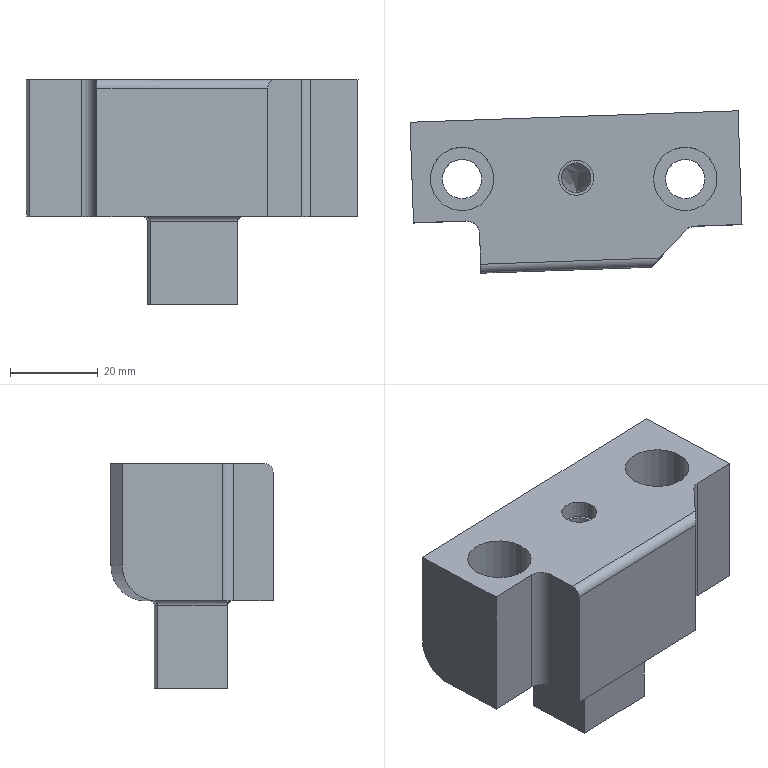Part | NX | features DIE-78 2 | 1 solid | 33 faces | box 75.862 x 37.072 x 51.4 mm | volume 69934 mm3 | plane 18 | cylinder 14 | cone 1 | commonest cylinder face diameters 2 x4 6 x2 9 x2 14.5 x2 4 x1 6.806 x1
STEP:
#1=CARTESIAN_POINT('',(3783.039,-805.598,860.616));
#2=VERTEX_POINT('',#1);
#3=CARTESIAN_POINT('',(3783.284,-812.594,860.616));
#4=VERTEX_POINT('',#3);
#5=CARTESIAN_POINT('',(3784.202,-838.885,860.616));
#6=DIRECTION('',(-0.0349,0.9994,0.));
#7=VECTOR('',#6,1000.);
#8=LINE('',#5,#7);
#9=EDGE_CURVE('',#2,#4,#8,.F.);
#10=ORIENTED_EDGE('',*,*,#9,.T.);
#11=CARTESIAN_POINT('',(3824.259,-811.163,860.616));
#12=VERTEX_POINT('',#11);
#13=CARTESIAN_POINT('',(3833.719,-810.833,860.616));
#14=DIRECTION('',(-0.9994,-0.0349,0.));
#15=VECTOR('',#14,1000.);
#16=LINE('',#13,#15);
#17=EDGE_CURVE('',#4,#12,#16,.F.);
#18=ORIENTED_EDGE('',*,*,#17,.T.);
#19=CARTESIAN_POINT('',(3830.163,-804.832,860.616));
#20=VERTEX_POINT('',#19);
#21=CARTESIAN_POINT('',(3816.137,-819.872,860.616));
#22=DIRECTION('',(0.682,0.7314,0.));
#23=VECTOR('',#22,1000.);
#24=LINE('',#21,#23);
#25=EDGE_CURVE('',#12,#20,#24,.T.);
#26=ORIENTED_EDGE('',*,*,#25,.T.);
#27=CARTESIAN_POINT('',(3832.252,-803.88,860.616));
#28=VERTEX_POINT('',#27);
#29=CARTESIAN_POINT('',(3832.357,-806.878,860.616));
#30=DIRECTION('',(0.,0.,-1.));
#31=DIRECTION('',(-1.,0.,0.));
#32=AXIS2_PLACEMENT_3D('',#29,#30,#31);
#33=CIRCLE('',#32,3.);
#34=EDGE_CURVE('',#20,#28,#33,.T.);
#35=ORIENTED_EDGE('',*,*,#34,.T.);
#36=CARTESIAN_POINT('',(3843.003,-803.505,860.616));
#37=VERTEX_POINT('',#36);
#38=CARTESIAN_POINT('',(3833.475,-803.837,860.616));
#39=DIRECTION('',(-0.9994,-0.0349,0.));
#40=VECTOR('',#39,1000.);
#41=LINE('',#38,#40);
#42=EDGE_CURVE('',#28,#37,#41,.F.);
#43=ORIENTED_EDGE('',*,*,#42,.T.);
#44=CARTESIAN_POINT('',(3842.096,-777.521,860.616));
#45=VERTEX_POINT('',#44);
#46=CARTESIAN_POINT('',(3842.011,-775.091,860.616));
#47=DIRECTION('',(0.0349,-0.9994,0.));
#48=VECTOR('',#47,1000.);
#49=LINE('',#46,#48);
#50=EDGE_CURVE('',#37,#45,#49,.F.);
#51=ORIENTED_EDGE('',*,*,#50,.T.);
#52=CARTESIAN_POINT('',(3767.141,-780.138,860.616));
#53=VERTEX_POINT('',#52);
#54=CARTESIAN_POINT('',(3832.568,-777.853,860.616));
#55=DIRECTION('',(-0.9994,-0.0349,0.));
#56=VECTOR('',#55,1000.);
#57=LINE('',#54,#56);
#58=EDGE_CURVE('',#53,#45,#57,.F.);
#59=ORIENTED_EDGE('',*,*,#58,.F.);
#60=CARTESIAN_POINT('',(3767.944,-803.124,860.616));
#61=VERTEX_POINT('',#60);
#62=CARTESIAN_POINT('',(3767.056,-777.709,860.616));
#63=DIRECTION('',(-0.0349,0.9994,0.));
#64=VECTOR('',#63,1000.);
#65=LINE('',#62,#64);
#66=EDGE_CURVE('',#53,#61,#65,.F.);
#67=ORIENTED_EDGE('',*,*,#66,.T.);
#68=CARTESIAN_POINT('',(3779.937,-802.705,860.616));
#69=VERTEX_POINT('',#68);
#70=CARTESIAN_POINT('',(3833.37,-800.839,860.616));
#71=DIRECTION('',(-0.9994,-0.0349,0.));
#72=VECTOR('',#71,1000.);
#73=LINE('',#70,#72);
#74=EDGE_CURVE('',#61,#69,#73,.F.);
#75=ORIENTED_EDGE('',*,*,#74,.T.);
#76=CARTESIAN_POINT('',(3780.041,-805.703,860.616));
#77=DIRECTION('',(0.,0.,-1.));
#78=DIRECTION('',(-1.,0.,0.));
#79=AXIS2_PLACEMENT_3D('',#76,#77,#78);
#80=CIRCLE('',#79,3.);
#81=EDGE_CURVE('',#69,#2,#80,.T.);
#82=ORIENTED_EDGE('',*,*,#81,.T.);
#83=EDGE_LOOP('',(#10,#18,#26,#35,#43,#51,#59,#67,#75,#82));
#84=FACE_BOUND('',#83,.T.);
#85=CARTESIAN_POINT('',(3771.787,-793.095,860.616));
#86=VERTEX_POINT('',#85);
#87=CARTESIAN_POINT('',(3779.037,-793.095,860.616));
#88=DIRECTION('',(0.,0.,-1.));
#89=DIRECTION('',(-1.,0.,0.));
#90=AXIS2_PLACEMENT_3D('',#87,#88,#89);
#91=CIRCLE('',#90,7.25);
#92=EDGE_CURVE('',#86,#86,#91,.F.);
#93=ORIENTED_EDGE('',*,*,#92,.F.);
#94=EDGE_LOOP('',(#93));
#95=FACE_BOUND('',#94,.T.);
#96=CARTESIAN_POINT('',(3822.787,-793.095,860.616));
#97=VERTEX_POINT('',#96);
#98=CARTESIAN_POINT('',(3830.037,-793.095,860.616));
#99=DIRECTION('',(0.,0.,-1.));
#100=DIRECTION('',(-1.,0.,0.));
#101=AXIS2_PLACEMENT_3D('',#98,#99,#100);
#102=CIRCLE('',#101,7.25);
#103=EDGE_CURVE('',#97,#97,#102,.F.);
#104=ORIENTED_EDGE('',*,*,#103,.F.);
#105=EDGE_LOOP('',(#104));
#106=FACE_BOUND('',#105,.T.);
#107=CARTESIAN_POINT('',(3809.107,-792.821,860.616));
#108=VERTEX_POINT('',#107);
#109=CARTESIAN_POINT('',(3805.107,-792.821,860.616));
#110=DIRECTION('',(0.,0.,-1.));
#111=DIRECTION('',(1.,0.,0.));
#112=AXIS2_PLACEMENT_3D('',#109,#110,#111);
#113=CIRCLE('',#112,4.);
#114=EDGE_CURVE('',#108,#108,#113,.T.);
#115=ORIENTED_EDGE('',*,*,#114,.T.);
#116=EDGE_LOOP('',(#115));
#117=FACE_BOUND('',#116,.T.);
#118=CARTESIAN_POINT('',(3834.637,-837.124,860.616));
#119=DIRECTION('',(0.,0.,-1.));
#120=DIRECTION('',(0.,-1.,0.));
#121=AXIS2_PLACEMENT_3D('',#118,#119,#120);
#122=PLANE('',#121);
#123=ADVANCED_FACE('',(#84,#95,#106,#117),#122,.F.);
#124=CARTESIAN_POINT('',(3767.42,-788.133,829.216));
#125=VERTEX_POINT('',#124);
#126=CARTESIAN_POINT('',(3767.141,-780.138,837.216));
#127=VERTEX_POINT('',#126);
#128=CARTESIAN_POINT('',(3767.42,-788.133,837.216));
#129=DIRECTION('',(0.9994,0.0349,0.000000002));
#130=DIRECTION('',(-0.0349,0.9994,0.));
#131=AXIS2_PLACEMENT_3D('',#128,#129,#130);
#132=CIRCLE('',#131,8.);
#133=EDGE_CURVE('',#125,#127,#132,.T.);
#134=ORIENTED_EDGE('',*,*,#133,.T.);
#135=CARTESIAN_POINT('',(3842.096,-777.521,837.216));
#136=VERTEX_POINT('',#135);
#137=CARTESIAN_POINT('',(3827.105,-778.044,837.216));
#138=DIRECTION('',(0.9994,0.0349,0.));
#139=VECTOR('',#138,1000.);
#140=LINE('',#137,#139);
#141=EDGE_CURVE('',#127,#136,#140,.T.);
#142=ORIENTED_EDGE('',*,*,#141,.T.);
#143=CARTESIAN_POINT('',(3842.375,-785.516,829.216));
#144=VERTEX_POINT('',#143);
#145=CARTESIAN_POINT('',(3842.375,-785.516,837.216));
#146=DIRECTION('',(-0.9994,-0.0349,-0.000000002));
#147=DIRECTION('',(0.0349,-0.9994,0.));
#148=AXIS2_PLACEMENT_3D('',#145,#146,#147);
#149=CIRCLE('',#148,8.);
#150=EDGE_CURVE('',#136,#144,#149,.T.);
#151=ORIENTED_EDGE('',*,*,#150,.T.);
#152=CARTESIAN_POINT('',(3815.891,-786.44,829.216));
#153=VERTEX_POINT('',#152);
#154=CARTESIAN_POINT('',(3782.411,-787.609,829.216));
#155=DIRECTION('',(0.9994,0.0349,0.));
#156=VECTOR('',#155,1000.);
#157=LINE('',#154,#156);
#158=EDGE_CURVE('',#153,#144,#157,.T.);
#159=ORIENTED_EDGE('',*,*,#158,.F.);
#160=CARTESIAN_POINT('',(3793.904,-787.208,829.216));
#161=VERTEX_POINT('',#160);
#162=CARTESIAN_POINT('',(3782.411,-787.609,829.216));
#163=DIRECTION('',(0.9994,0.0349,0.));
#164=VECTOR('',#163,1000.);
#165=LINE('',#162,#164);
#166=EDGE_CURVE('',#161,#153,#165,.T.);
#167=ORIENTED_EDGE('',*,*,#166,.F.);
#168=CARTESIAN_POINT('',(3782.411,-787.609,829.216));
#169=DIRECTION('',(0.9994,0.0349,0.));
#170=VECTOR('',#169,1000.);
#171=LINE('',#168,#170);
#172=EDGE_CURVE('',#125,#161,#171,.T.);
#173=ORIENTED_EDGE('',*,*,#172,.F.);
#174=EDGE_LOOP('',(#134,#142,#151,#159,#167,#173));
#175=FACE_BOUND('',#174,.T.);
#176=CARTESIAN_POINT('',(3782.411,-787.609,837.216));
#177=DIRECTION('',(0.9994,0.0349,0.000000002));
#178=DIRECTION('',(-0.0349,0.9994,0.));
#179=AXIS2_PLACEMENT_3D('',#176,#177,#178);
#180=CYLINDRICAL_SURFACE('',#179,8.);
#181=ADVANCED_FACE('',(#175),#180,.T.);
#182=ORIENTED_EDGE('',*,*,#81,.F.);
#183=CARTESIAN_POINT('',(3779.937,-802.705,829.216));
#184=VERTEX_POINT('',#183);
#185=CARTESIAN_POINT('',(3779.937,-802.705,860.616));
#186=DIRECTION('',(0.,0.000000057,-1.));
#187=VECTOR('',#186,1000.);
#188=LINE('',#185,#187);
#189=EDGE_CURVE('',#184,#69,#188,.F.);
#190=ORIENTED_EDGE('',*,*,#189,.F.);
#191=CARTESIAN_POINT('',(3783.039,-805.598,829.216));
#192=VERTEX_POINT('',#191);
#193=CARTESIAN_POINT('',(3780.041,-805.703,829.216));
#194=DIRECTION('',(0.,0.,-1.));
#195=DIRECTION('',(-1.,0.,0.));
#196=AXIS2_PLACEMENT_3D('',#193,#194,#195);
#197=CIRCLE('',#196,3.);
#198=EDGE_CURVE('',#192,#184,#197,.F.);
#199=ORIENTED_EDGE('',*,*,#198,.F.);
#200=CARTESIAN_POINT('',(3783.039,-805.598,829.216));
#201=DIRECTION('',(0.,0.000000057,-1.));
#202=VECTOR('',#201,1000.);
#203=LINE('',#200,#202);
#204=EDGE_CURVE('',#2,#192,#203,.T.);
#205=ORIENTED_EDGE('',*,*,#204,.F.);
#206=EDGE_LOOP('',(#182,#190,#199,#205));
#207=FACE_BOUND('',#206,.T.);
#208=CARTESIAN_POINT('',(3780.041,-805.703,842.216));
#209=DIRECTION('',(0.,-0.000000057,1.));
#210=DIRECTION('',(0.,-1.,-0.000000057));
#211=AXIS2_PLACEMENT_3D('',#208,#209,#210);
#212=CYLINDRICAL_SURFACE('',#211,3.);
#213=ADVANCED_FACE('',(#207),#212,.F.);
#214=CARTESIAN_POINT('',(3767.944,-803.124,829.216));
#215=VERTEX_POINT('',#214);
#216=CARTESIAN_POINT('',(3040.928,-828.509,829.216));
#217=DIRECTION('',(-0.9994,-0.0349,0.));
#218=VECTOR('',#217,1000.);
#219=LINE('',#216,#218);
#220=EDGE_CURVE('',#184,#215,#219,.T.);
#221=ORIENTED_EDGE('',*,*,#220,.F.);
#222=ORIENTED_EDGE('',*,*,#189,.T.);
#223=ORIENTED_EDGE('',*,*,#74,.F.);
#224=CARTESIAN_POINT('',(3767.944,-803.124,842.216));
#225=DIRECTION('',(0.,-0.000000057,1.));
#226=VECTOR('',#225,1000.);
#227=LINE('',#224,#226);
#228=EDGE_CURVE('',#215,#61,#227,.T.);
#229=ORIENTED_EDGE('',*,*,#228,.F.);
#230=EDGE_LOOP('',(#221,#222,#223,#229));
#231=FACE_BOUND('',#230,.T.);
#232=CARTESIAN_POINT('',(3835.403,-800.768,844.916));
#233=DIRECTION('',(0.0349,-0.9994,-0.000000057));
#234=DIRECTION('',(0.9994,0.0349,0.));
#235=AXIS2_PLACEMENT_3D('',#232,#233,#234);
#236=PLANE('',#235);
#237=ADVANCED_FACE('',(#231),#236,.T.);
#238=CARTESIAN_POINT('',(3767.056,-777.709,829.216));
#239=DIRECTION('',(-0.0349,0.9994,0.));
#240=VECTOR('',#239,1000.);
#241=LINE('',#238,#240);
#242=EDGE_CURVE('',#125,#215,#241,.F.);
#243=ORIENTED_EDGE('',*,*,#242,.T.);
#244=ORIENTED_EDGE('',*,*,#228,.T.);
#245=ORIENTED_EDGE('',*,*,#66,.F.);
#246=CARTESIAN_POINT('',(3767.141,-780.138,823.716));
#247=DIRECTION('',(0.,-0.000000057,1.));
#248=VECTOR('',#247,1000.);
#249=LINE('',#246,#248);
#250=EDGE_CURVE('',#127,#53,#249,.T.);
#251=ORIENTED_EDGE('',*,*,#250,.F.);
#252=ORIENTED_EDGE('',*,*,#133,.F.);
#253=EDGE_LOOP('',(#243,#244,#245,#251,#252));
#254=FACE_BOUND('',#253,.T.);
#255=CARTESIAN_POINT('',(3767.056,-777.709,842.216));
#256=DIRECTION('',(-0.9994,-0.0349,-0.000000002));
#257=DIRECTION('',(-0.0349,0.9994,0.));
#258=AXIS2_PLACEMENT_3D('',#255,#256,#257);
#259=PLANE('',#258);
#260=ADVANCED_FACE('',(#254),#259,.T.);
#261=ORIENTED_EDGE('',*,*,#141,.F.);
#262=ORIENTED_EDGE('',*,*,#250,.T.);
#263=ORIENTED_EDGE('',*,*,#58,.T.);
#264=CARTESIAN_POINT('',(3842.096,-777.521,823.716));
#265=DIRECTION('',(0.,0.000000057,-1.));
#266=VECTOR('',#265,1000.);
#267=LINE('',#264,#266);
#268=EDGE_CURVE('',#45,#136,#267,.T.);
#269=ORIENTED_EDGE('',*,*,#268,.T.);
#270=EDGE_LOOP('',(#261,#262,#263,#269));
#271=FACE_BOUND('',#270,.T.);
#272=CARTESIAN_POINT('',(3789.628,-779.353,823.716));
#273=DIRECTION('',(0.0349,-0.9994,-0.000000057));
#274=DIRECTION('',(-0.9994,-0.0349,0.));
#275=AXIS2_PLACEMENT_3D('',#272,#273,#274);
#276=PLANE('',#275);
#277=ADVANCED_FACE('',(#271),#276,.F.);
#278=ORIENTED_EDGE('',*,*,#50,.F.);
#279=CARTESIAN_POINT('',(3843.003,-803.505,829.216));
#280=VERTEX_POINT('',#279);
#281=CARTESIAN_POINT('',(3843.003,-803.505,842.216));
#282=DIRECTION('',(0.,0.000000057,-1.));
#283=VECTOR('',#282,1000.);
#284=LINE('',#281,#283);
#285=EDGE_CURVE('',#37,#280,#284,.T.);
#286=ORIENTED_EDGE('',*,*,#285,.T.);
#287=CARTESIAN_POINT('',(3842.011,-775.091,829.216));
#288=DIRECTION('',(0.0349,-0.9994,0.));
#289=VECTOR('',#288,1000.);
#290=LINE('',#287,#289);
#291=EDGE_CURVE('',#280,#144,#290,.F.);
#292=ORIENTED_EDGE('',*,*,#291,.T.);
#293=ORIENTED_EDGE('',*,*,#150,.F.);
#294=ORIENTED_EDGE('',*,*,#268,.F.);
#295=EDGE_LOOP('',(#278,#286,#292,#293,#294));
#296=FACE_BOUND('',#295,.T.);
#297=CARTESIAN_POINT('',(3842.011,-775.091,842.216));
#298=DIRECTION('',(0.9994,0.0349,0.000000002));
#299=DIRECTION('',(0.0349,-0.9994,0.));
#300=AXIS2_PLACEMENT_3D('',#297,#298,#299);
#301=PLANE('',#300);
#302=ADVANCED_FACE('',(#296),#301,.T.);
#303=ORIENTED_EDGE('',*,*,#42,.F.);
#304=CARTESIAN_POINT('',(3832.252,-803.88,829.216));
#305=VERTEX_POINT('',#304);
#306=CARTESIAN_POINT('',(3832.252,-803.88,829.216));
#307=DIRECTION('',(0.,-0.000000057,1.));
#308=VECTOR('',#307,1000.);
#309=LINE('',#306,#308);
#310=EDGE_CURVE('',#28,#305,#309,.F.);
#311=ORIENTED_EDGE('',*,*,#310,.T.);
#312=CARTESIAN_POINT('',(3828.012,-804.028,829.216));
#313=DIRECTION('',(0.9994,0.0349,0.));
#314=VECTOR('',#313,1000.);
#315=LINE('',#312,#314);
#316=EDGE_CURVE('',#305,#280,#315,.T.);
#317=ORIENTED_EDGE('',*,*,#316,.T.);
#318=ORIENTED_EDGE('',*,*,#285,.F.);
#319=EDGE_LOOP('',(#303,#311,#317,#318));
#320=FACE_BOUND('',#319,.T.);
#321=CARTESIAN_POINT('',(3828.012,-804.028,842.216));
#322=DIRECTION('',(0.0349,-0.9994,-0.000000057));
#323=DIRECTION('',(0.,0.000000057,-1.));
#324=AXIS2_PLACEMENT_3D('',#321,#322,#323);
#325=PLANE('',#324);
#326=ADVANCED_FACE('',(#320),#325,.T.);
#327=ORIENTED_EDGE('',*,*,#34,.F.);
#328=CARTESIAN_POINT('',(3830.163,-804.832,829.216));
#329=VERTEX_POINT('',#328);
#330=CARTESIAN_POINT('',(3830.163,-804.832,860.616));
#331=DIRECTION('',(0.,0.000000057,-1.));
#332=VECTOR('',#331,1000.);
#333=LINE('',#330,#332);
#334=EDGE_CURVE('',#329,#20,#333,.F.);
#335=ORIENTED_EDGE('',*,*,#334,.F.);
#336=CARTESIAN_POINT('',(3832.357,-806.878,829.216));
#337=DIRECTION('',(0.,0.,-1.));
#338=DIRECTION('',(-1.,0.,0.));
#339=AXIS2_PLACEMENT_3D('',#336,#337,#338);
#340=CIRCLE('',#339,3.);
#341=EDGE_CURVE('',#305,#329,#340,.F.);
#342=ORIENTED_EDGE('',*,*,#341,.F.);
#343=ORIENTED_EDGE('',*,*,#310,.F.);
#344=EDGE_LOOP('',(#327,#335,#342,#343));
#345=FACE_BOUND('',#344,.T.);
#346=CARTESIAN_POINT('',(3832.357,-806.878,842.216));
#347=DIRECTION('',(0.,0.000000057,-1.));
#348=DIRECTION('',(0.,1.,0.000000057));
#349=AXIS2_PLACEMENT_3D('',#346,#347,#348);
#350=CYLINDRICAL_SURFACE('',#349,3.);
#351=ADVANCED_FACE('',(#345),#350,.F.);
#352=CARTESIAN_POINT('',(3825.537,-793.095,829.216));
#353=VERTEX_POINT('',#352);
#354=CARTESIAN_POINT('',(3830.037,-793.095,829.216));
#355=DIRECTION('',(0.,0.,-1.));
#356=DIRECTION('',(-1.,0.,0.));
#357=AXIS2_PLACEMENT_3D('',#354,#355,#356);
#358=CIRCLE('',#357,4.5);
#359=EDGE_CURVE('',#353,#353,#358,.T.);
#360=ORIENTED_EDGE('',*,*,#359,.F.);
#361=EDGE_LOOP('',(#360));
#362=FACE_BOUND('',#361,.T.);
#363=CARTESIAN_POINT('',(3774.537,-793.095,829.216));
#364=VERTEX_POINT('',#363);
#365=CARTESIAN_POINT('',(3779.037,-793.095,829.216));
#366=DIRECTION('',(0.,0.,-1.));
#367=DIRECTION('',(-1.,0.,0.));
#368=AXIS2_PLACEMENT_3D('',#365,#366,#367);
#369=CIRCLE('',#368,4.5);
#370=EDGE_CURVE('',#364,#364,#369,.T.);
#371=ORIENTED_EDGE('',*,*,#370,.F.);
#372=EDGE_LOOP('',(#371));
#373=FACE_BOUND('',#372,.T.);
#374=CARTESIAN_POINT('',(3794.532,-805.197,829.216));
#375=VERTEX_POINT('',#374);
#376=CARTESIAN_POINT('',(3816.519,-804.429,829.216));
#377=VERTEX_POINT('',#376);
#378=CARTESIAN_POINT('',(3815.52,-804.464,829.216));
#379=DIRECTION('',(-0.9994,-0.0349,0.));
#380=VECTOR('',#379,1000.);
#381=LINE('',#378,#380);
#382=EDGE_CURVE('',#375,#377,#381,.F.);
#383=ORIENTED_EDGE('',*,*,#382,.T.);
#384=CARTESIAN_POINT('',(3815.682,-780.462,829.216));
#385=DIRECTION('',(-0.0349,0.9994,0.));
#386=VECTOR('',#385,1000.);
#387=LINE('',#384,#386);
#388=EDGE_CURVE('',#377,#153,#387,.T.);
#389=ORIENTED_EDGE('',*,*,#388,.T.);
#390=ORIENTED_EDGE('',*,*,#158,.T.);
#391=ORIENTED_EDGE('',*,*,#291,.F.);
#392=ORIENTED_EDGE('',*,*,#316,.F.);
#393=ORIENTED_EDGE('',*,*,#341,.T.);
#394=CARTESIAN_POINT('',(3822.33,-813.232,829.216));
#395=VERTEX_POINT('',#394);
#396=CARTESIAN_POINT('',(3461.379,-1200.302,829.216));
#397=DIRECTION('',(0.682,0.7314,0.));
#398=VECTOR('',#397,1000.);
#399=LINE('',#396,#398);
#400=EDGE_CURVE('',#329,#395,#399,.F.);
#401=ORIENTED_EDGE('',*,*,#400,.T.);
#402=CARTESIAN_POINT('',(3783.353,-814.593,829.216));
#403=VERTEX_POINT('',#402);
#404=CARTESIAN_POINT('',(3843.369,-812.497,829.216));
#405=DIRECTION('',(-0.9994,-0.0349,0.));
#406=VECTOR('',#405,1000.);
#407=LINE('',#404,#406);
#408=EDGE_CURVE('',#395,#403,#407,.T.);
#409=ORIENTED_EDGE('',*,*,#408,.T.);
#410=CARTESIAN_POINT('',(3782.203,-781.631,829.216));
#411=DIRECTION('',(0.0349,-0.9994,0.));
#412=VECTOR('',#411,1000.);
#413=LINE('',#410,#412);
#414=EDGE_CURVE('',#192,#403,#413,.T.);
#415=ORIENTED_EDGE('',*,*,#414,.F.);
#416=ORIENTED_EDGE('',*,*,#198,.T.);
#417=ORIENTED_EDGE('',*,*,#220,.T.);
#418=ORIENTED_EDGE('',*,*,#242,.F.);
#419=ORIENTED_EDGE('',*,*,#172,.T.);
#420=CARTESIAN_POINT('',(3794.498,-804.198,829.216));
#421=DIRECTION('',(-0.0349,0.9994,0.));
#422=VECTOR('',#421,1000.);
#423=LINE('',#420,#422);
#424=EDGE_CURVE('',#161,#375,#423,.F.);
#425=ORIENTED_EDGE('',*,*,#424,.T.);
#426=EDGE_LOOP('',(#383,#389,#390,#391,#392,#393,#401,#409,#415,#416,#417,#418,#419,#425));
#427=FACE_BOUND('',#426,.T.);
#428=CARTESIAN_POINT('',(3040.196,-807.539,829.216));
#429=DIRECTION('',(0.,0.,-1.));
#430=DIRECTION('',(0.0349,-0.9994,0.));
#431=AXIS2_PLACEMENT_3D('',#428,#429,#430);
#432=PLANE('',#431);
#433=ADVANCED_FACE('',(#362,#373,#427),#432,.T.);
#434=ORIENTED_EDGE('',*,*,#25,.F.);
#435=CARTESIAN_POINT('',(3822.33,-813.232,858.616));
#436=VERTEX_POINT('',#435);
#437=CARTESIAN_POINT('',(3824.259,-811.163,858.616));
#438=DIRECTION('',(-0.7314,0.682,0.000000039));
#439=DIRECTION('',(0.682,0.7314,0.000000039));
#440=AXIS2_PLACEMENT_3D('',#437,#438,#439);
#441=ELLIPSE('',#440,2.828,2.);
#442=EDGE_CURVE('',#12,#436,#441,.F.);
#443=ORIENTED_EDGE('',*,*,#442,.T.);
#444=CARTESIAN_POINT('',(3822.33,-813.232,854.74));
#445=DIRECTION('',(0.,-0.000000057,1.));
#446=VECTOR('',#445,1000.);
#447=LINE('',#444,#446);
#448=EDGE_CURVE('',#395,#436,#447,.T.);
#449=ORIENTED_EDGE('',*,*,#448,.F.);
#450=ORIENTED_EDGE('',*,*,#400,.F.);
#451=ORIENTED_EDGE('',*,*,#334,.T.);
#452=EDGE_LOOP('',(#434,#443,#449,#450,#451));
#453=FACE_BOUND('',#452,.T.);
#454=CARTESIAN_POINT('',(3822.33,-813.232,854.74));
#455=DIRECTION('',(-0.7314,0.682,0.000000039));
#456=DIRECTION('',(0.,-0.000000057,1.));
#457=AXIS2_PLACEMENT_3D('',#454,#455,#456);
#458=PLANE('',#457);
#459=ADVANCED_FACE('',(#453),#458,.F.);
#460=CARTESIAN_POINT('',(3783.353,-814.593,858.616));
#461=VERTEX_POINT('',#460);
#462=CARTESIAN_POINT('',(3783.353,-814.593,842.216));
#463=DIRECTION('',(0.,0.000000057,-1.));
#464=VECTOR('',#463,1000.);
#465=LINE('',#462,#464);
#466=EDGE_CURVE('',#461,#403,#465,.T.);
#467=ORIENTED_EDGE('',*,*,#466,.F.);
#468=CARTESIAN_POINT('',(3783.284,-812.594,858.616));
#469=DIRECTION('',(-0.9994,-0.0349,-0.000000002));
#470=DIRECTION('',(0.0349,-0.9994,0.));
#471=AXIS2_PLACEMENT_3D('',#468,#469,#470);
#472=CIRCLE('',#471,2.);
#473=EDGE_CURVE('',#461,#4,#472,.T.);
#474=ORIENTED_EDGE('',*,*,#473,.T.);
#475=ORIENTED_EDGE('',*,*,#9,.F.);
#476=ORIENTED_EDGE('',*,*,#204,.T.);
#477=ORIENTED_EDGE('',*,*,#414,.T.);
#478=EDGE_LOOP('',(#467,#474,#475,#476,#477));
#479=FACE_BOUND('',#478,.T.);
#480=CARTESIAN_POINT('',(3782.047,-777.185,842.216));
#481=DIRECTION('',(-0.9994,-0.0349,-0.000000002));
#482=DIRECTION('',(-0.0349,0.9994,0.));
#483=AXIS2_PLACEMENT_3D('',#480,#481,#482);
#484=PLANE('',#483);
#485=ADVANCED_FACE('',(#479),#484,.T.);
#486=ORIENTED_EDGE('',*,*,#448,.T.);
#487=CARTESIAN_POINT('',(3843.369,-812.497,858.616));
#488=DIRECTION('',(0.9994,0.0349,0.));
#489=VECTOR('',#488,1000.);
#490=LINE('',#487,#489);
#491=EDGE_CURVE('',#436,#461,#490,.F.);
#492=ORIENTED_EDGE('',*,*,#491,.T.);
#493=ORIENTED_EDGE('',*,*,#466,.T.);
#494=ORIENTED_EDGE('',*,*,#408,.F.);
#495=EDGE_LOOP('',(#486,#492,#493,#494));
#496=FACE_BOUND('',#495,.T.);
#497=CARTESIAN_POINT('',(3843.369,-812.497,854.74));
#498=DIRECTION('',(0.0349,-0.9994,-0.000000057));
#499=DIRECTION('',(0.,-0.000000057,1.));
#500=AXIS2_PLACEMENT_3D('',#497,#498,#499);
#501=PLANE('',#500);
#502=ADVANCED_FACE('',(#496),#501,.T.);
#503=ORIENTED_EDGE('',*,*,#442,.F.);
#504=ORIENTED_EDGE('',*,*,#17,.F.);
#505=ORIENTED_EDGE('',*,*,#473,.F.);
#506=ORIENTED_EDGE('',*,*,#491,.F.);
#507=EDGE_LOOP('',(#503,#504,#505,#506));
#508=FACE_BOUND('',#507,.T.);
#509=CARTESIAN_POINT('',(3843.299,-810.499,858.616));
#510=DIRECTION('',(0.9994,0.0349,0.));
#511=DIRECTION('',(-0.0349,0.9994,0.));
#512=AXIS2_PLACEMENT_3D('',#509,#510,#511);
#513=CYLINDRICAL_SURFACE('',#512,2.);
#514=ADVANCED_FACE('',(#508),#513,.T.);
#515=CARTESIAN_POINT('',(3814.926,-787.475,809.216));
#516=VERTEX_POINT('',#515);
#517=CARTESIAN_POINT('',(3794.939,-788.173,809.216));
#518=VERTEX_POINT('',#517);
#519=CARTESIAN_POINT('',(3804.932,-787.824,809.216));
#520=DIRECTION('',(0.9994,0.0349,0.));
#521=VECTOR('',#520,1000.);
#522=LINE('',#519,#521);
#523=EDGE_CURVE('',#516,#518,#522,.F.);
#524=ORIENTED_EDGE('',*,*,#523,.F.);
#525=CARTESIAN_POINT('',(3815.485,-803.465,809.216));
#526=VERTEX_POINT('',#525);
#527=CARTESIAN_POINT('',(3815.485,-803.465,809.216));
#528=DIRECTION('',(-0.0349,0.9994,0.));
#529=VECTOR('',#528,1000.);
#530=LINE('',#527,#529);
#531=EDGE_CURVE('',#516,#526,#530,.F.);
#532=ORIENTED_EDGE('',*,*,#531,.T.);
#533=CARTESIAN_POINT('',(3795.497,-804.163,809.216));
#534=VERTEX_POINT('',#533);
#535=CARTESIAN_POINT('',(3805.491,-803.814,809.216));
#536=DIRECTION('',(0.9994,0.0349,0.));
#537=VECTOR('',#536,1000.);
#538=LINE('',#535,#537);
#539=EDGE_CURVE('',#526,#534,#538,.F.);
#540=ORIENTED_EDGE('',*,*,#539,.T.);
#541=CARTESIAN_POINT('',(3795.497,-804.163,809.216));
#542=DIRECTION('',(-0.0349,0.9994,0.));
#543=VECTOR('',#542,1000.);
#544=LINE('',#541,#543);
#545=EDGE_CURVE('',#518,#534,#544,.F.);
#546=ORIENTED_EDGE('',*,*,#545,.F.);
#547=EDGE_LOOP('',(#524,#532,#540,#546));
#548=FACE_BOUND('',#547,.T.);
#549=CARTESIAN_POINT('',(3804.689,-780.846,809.216));
#550=DIRECTION('',(0.,0.,1.));
#551=DIRECTION('',(-0.0349,0.9994,0.));
#552=AXIS2_PLACEMENT_3D('',#549,#550,#551);
#553=PLANE('',#552);
#554=ADVANCED_FACE('',(#548),#553,.F.);
#555=CARTESIAN_POINT('',(3815.485,-803.465,828.216));
#556=VERTEX_POINT('',#555);
#557=CARTESIAN_POINT('',(3815.485,-803.465,821.716));
#558=DIRECTION('',(0.,0.,-1.));
#559=VECTOR('',#558,1000.);
#560=LINE('',#557,#559);
#561=EDGE_CURVE('',#556,#526,#560,.T.);
#562=ORIENTED_EDGE('',*,*,#561,.F.);
#563=CARTESIAN_POINT('',(3795.497,-804.163,828.216));
#564=VERTEX_POINT('',#563);
#565=CARTESIAN_POINT('',(3795.497,-804.163,828.216));
#566=DIRECTION('',(-0.9994,-0.0349,0.));
#567=VECTOR('',#566,1000.);
#568=LINE('',#565,#567);
#569=EDGE_CURVE('',#556,#564,#568,.T.);
#570=ORIENTED_EDGE('',*,*,#569,.T.);
#571=CARTESIAN_POINT('',(3795.497,-804.163,814.216));
#572=DIRECTION('',(0.,0.,1.));
#573=VECTOR('',#572,1000.);
#574=LINE('',#571,#573);
#575=EDGE_CURVE('',#564,#534,#574,.F.);
#576=ORIENTED_EDGE('',*,*,#575,.T.);
#577=ORIENTED_EDGE('',*,*,#539,.F.);
#578=EDGE_LOOP('',(#562,#570,#576,#577));
#579=FACE_BOUND('',#578,.T.);
#580=CARTESIAN_POINT('',(3805.491,-803.814,821.716));
#581=DIRECTION('',(0.0349,-0.9994,0.));
#582=DIRECTION('',(0.,0.,1.));
#583=AXIS2_PLACEMENT_3D('',#580,#581,#582);
#584=PLANE('',#583);
#585=ADVANCED_FACE('',(#579),#584,.T.);
#586=CARTESIAN_POINT('',(3794.939,-788.173,828.216));
#587=VERTEX_POINT('',#586);
#588=CARTESIAN_POINT('',(3794.939,-788.173,814.216));
#589=DIRECTION('',(0.,0.,1.));
#590=VECTOR('',#589,1000.);
#591=LINE('',#588,#590);
#592=EDGE_CURVE('',#518,#587,#591,.T.);
#593=ORIENTED_EDGE('',*,*,#592,.T.);
#594=CARTESIAN_POINT('',(3814.926,-787.475,828.216));
#595=VERTEX_POINT('',#594);
#596=CARTESIAN_POINT('',(3814.926,-787.475,828.216));
#597=DIRECTION('',(-0.9994,-0.0349,0.));
#598=VECTOR('',#597,1000.);
#599=LINE('',#596,#598);
#600=EDGE_CURVE('',#587,#595,#599,.F.);
#601=ORIENTED_EDGE('',*,*,#600,.T.);
#602=CARTESIAN_POINT('',(3814.926,-787.475,814.216));
#603=DIRECTION('',(0.,0.,1.));
#604=VECTOR('',#603,1000.);
#605=LINE('',#602,#604);
#606=EDGE_CURVE('',#516,#595,#605,.T.);
#607=ORIENTED_EDGE('',*,*,#606,.F.);
#608=ORIENTED_EDGE('',*,*,#523,.T.);
#609=EDGE_LOOP('',(#593,#601,#607,#608));
#610=FACE_BOUND('',#609,.T.);
#611=CARTESIAN_POINT('',(3804.932,-787.824,814.216));
#612=DIRECTION('',(-0.0349,0.9994,0.));
#613=DIRECTION('',(0.,0.,-1.));
#614=AXIS2_PLACEMENT_3D('',#611,#612,#613);
#615=PLANE('',#614);
#616=ADVANCED_FACE('',(#610),#615,.T.);
#617=ORIENTED_EDGE('',*,*,#575,.F.);
#618=CARTESIAN_POINT('',(3794.904,-787.173,828.216));
#619=DIRECTION('',(-0.0349,0.9994,0.));
#620=VECTOR('',#619,1000.);
#621=LINE('',#618,#620);
#622=EDGE_CURVE('',#564,#587,#621,.T.);
#623=ORIENTED_EDGE('',*,*,#622,.T.);
#624=ORIENTED_EDGE('',*,*,#592,.F.);
#625=ORIENTED_EDGE('',*,*,#545,.T.);
#626=EDGE_LOOP('',(#617,#623,#624,#625));
#627=FACE_BOUND('',#626,.T.);
#628=CARTESIAN_POINT('',(3795.497,-804.163,814.216));
#629=DIRECTION('',(-0.9994,-0.0349,0.));
#630=DIRECTION('',(0.0349,-0.9994,0.));
#631=AXIS2_PLACEMENT_3D('',#628,#629,#630);
#632=PLANE('',#631);
#633=ADVANCED_FACE('',(#627),#632,.T.);
#634=ORIENTED_EDGE('',*,*,#606,.T.);
#635=CARTESIAN_POINT('',(3815.485,-803.465,828.216));
#636=DIRECTION('',(-0.0349,0.9994,0.));
#637=VECTOR('',#636,1000.);
#638=LINE('',#635,#637);
#639=EDGE_CURVE('',#595,#556,#638,.F.);
#640=ORIENTED_EDGE('',*,*,#639,.T.);
#641=ORIENTED_EDGE('',*,*,#561,.T.);
#642=ORIENTED_EDGE('',*,*,#531,.F.);
#643=EDGE_LOOP('',(#634,#640,#641,#642));
#644=FACE_BOUND('',#643,.T.);
#645=CARTESIAN_POINT('',(3815.485,-803.465,814.216));
#646=DIRECTION('',(-0.9994,-0.0349,0.));
#647=DIRECTION('',(0.0349,-0.9994,0.));
#648=AXIS2_PLACEMENT_3D('',#645,#646,#647);
#649=PLANE('',#648);
#650=ADVANCED_FACE('',(#644),#649,.F.);
#651=ORIENTED_EDGE('',*,*,#166,.T.);
#652=CARTESIAN_POINT('',(3815.891,-786.44,828.216));
#653=DIRECTION('',(0.7314,-0.682,0.));
#654=DIRECTION('',(0.682,0.7314,0.));
#655=AXIS2_PLACEMENT_3D('',#652,#653,#654);
#656=ELLIPSE('',#655,1.414,1.);
#657=EDGE_CURVE('',#153,#595,#656,.T.);
#658=ORIENTED_EDGE('',*,*,#657,.T.);
#659=ORIENTED_EDGE('',*,*,#600,.F.);
#660=CARTESIAN_POINT('',(3793.904,-787.208,828.216));
#661=DIRECTION('',(0.682,0.7314,0.));
#662=DIRECTION('',(0.7314,-0.682,0.));
#663=AXIS2_PLACEMENT_3D('',#660,#661,#662);
#664=ELLIPSE('',#663,1.414,1.);
#665=EDGE_CURVE('',#587,#161,#664,.F.);
#666=ORIENTED_EDGE('',*,*,#665,.T.);
#667=EDGE_LOOP('',(#651,#658,#659,#666));
#668=FACE_BOUND('',#667,.T.);
#669=CARTESIAN_POINT('',(3040.405,-813.518,828.216));
#670=DIRECTION('',(0.9994,0.0349,0.));
#671=DIRECTION('',(-0.0349,0.9994,0.));
#672=AXIS2_PLACEMENT_3D('',#669,#670,#671);
#673=CYLINDRICAL_SURFACE('',#672,1.);
#674=ADVANCED_FACE('',(#668),#673,.F.);
#675=ORIENTED_EDGE('',*,*,#665,.F.);
#676=ORIENTED_EDGE('',*,*,#622,.F.);
#677=CARTESIAN_POINT('',(3794.532,-805.197,828.216));
#678=DIRECTION('',(0.7314,-0.682,0.));
#679=DIRECTION('',(-0.682,-0.7314,0.));
#680=AXIS2_PLACEMENT_3D('',#677,#678,#679);
#681=ELLIPSE('',#680,1.414,1.);
#682=EDGE_CURVE('',#375,#564,#681,.F.);
#683=ORIENTED_EDGE('',*,*,#682,.F.);
#684=ORIENTED_EDGE('',*,*,#424,.F.);
#685=EDGE_LOOP('',(#675,#676,#683,#684));
#686=FACE_BOUND('',#685,.T.);
#687=CARTESIAN_POINT('',(3794.498,-804.198,828.216));
#688=DIRECTION('',(0.0349,-0.9994,0.));
#689=DIRECTION('',(0.9994,0.0349,0.));
#690=AXIS2_PLACEMENT_3D('',#687,#688,#689);
#691=CYLINDRICAL_SURFACE('',#690,1.);
#692=ADVANCED_FACE('',(#686),#691,.F.);
#693=ORIENTED_EDGE('',*,*,#682,.T.);
#694=ORIENTED_EDGE('',*,*,#569,.F.);
#695=CARTESIAN_POINT('',(3816.519,-804.429,828.216));
#696=DIRECTION('',(0.682,0.7314,0.));
#697=DIRECTION('',(0.7314,-0.682,0.));
#698=AXIS2_PLACEMENT_3D('',#695,#696,#697);
#699=ELLIPSE('',#698,1.414,1.);
#700=EDGE_CURVE('',#377,#556,#699,.F.);
#701=ORIENTED_EDGE('',*,*,#700,.F.);
#702=ORIENTED_EDGE('',*,*,#382,.F.);
#703=EDGE_LOOP('',(#693,#694,#701,#702));
#704=FACE_BOUND('',#703,.T.);
#705=CARTESIAN_POINT('',(3805.526,-804.813,828.216));
#706=DIRECTION('',(0.9994,0.0349,0.));
#707=DIRECTION('',(-0.0349,0.9994,0.));
#708=AXIS2_PLACEMENT_3D('',#705,#706,#707);
#709=CYLINDRICAL_SURFACE('',#708,1.);
#710=ADVANCED_FACE('',(#704),#709,.F.);
#711=ORIENTED_EDGE('',*,*,#700,.T.);
#712=ORIENTED_EDGE('',*,*,#639,.F.);
#713=ORIENTED_EDGE('',*,*,#657,.F.);
#714=ORIENTED_EDGE('',*,*,#388,.F.);
#715=EDGE_LOOP('',(#711,#712,#713,#714));
#716=FACE_BOUND('',#715,.T.);
#717=CARTESIAN_POINT('',(3815.682,-780.462,828.216));
#718=DIRECTION('',(-0.0349,0.9994,0.));
#719=DIRECTION('',(-0.9994,-0.0349,0.));
#720=AXIS2_PLACEMENT_3D('',#717,#718,#719);
#721=CYLINDRICAL_SURFACE('',#720,1.);
#722=ADVANCED_FACE('',(#716),#721,.F.);
#723=ORIENTED_EDGE('',*,*,#370,.T.);
#724=EDGE_LOOP('',(#723));
#725=FACE_BOUND('',#724,.T.);
#726=CARTESIAN_POINT('',(3783.537,-793.095,847.616));
#727=VERTEX_POINT('',#726);
#728=CARTESIAN_POINT('',(3779.037,-793.095,847.616));
#729=DIRECTION('',(0.,0.,1.));
#730=DIRECTION('',(1.,0.,0.));
#731=AXIS2_PLACEMENT_3D('',#728,#729,#730);
#732=CIRCLE('',#731,4.5);
#733=EDGE_CURVE('',#727,#727,#732,.T.);
#734=ORIENTED_EDGE('',*,*,#733,.T.);
#735=EDGE_LOOP('',(#734));
#736=FACE_BOUND('',#735,.T.);
#737=CARTESIAN_POINT('',(3779.037,-793.095,808.216));
#738=DIRECTION('',(0.,0.,1.));
#739=DIRECTION('',(1.,0.,0.));
#740=AXIS2_PLACEMENT_3D('',#737,#738,#739);
#741=CYLINDRICAL_SURFACE('',#740,4.5);
#742=ADVANCED_FACE('',(#725,#736),#741,.F.);
#743=ORIENTED_EDGE('',*,*,#92,.T.);
#744=EDGE_LOOP('',(#743));
#745=FACE_BOUND('',#744,.T.);
#746=CARTESIAN_POINT('',(3786.287,-793.095,847.616));
#747=VERTEX_POINT('',#746);
#748=CARTESIAN_POINT('',(3779.037,-793.095,847.616));
#749=DIRECTION('',(0.,0.,1.));
#750=DIRECTION('',(1.,0.,0.));
#751=AXIS2_PLACEMENT_3D('',#748,#749,#750);
#752=CIRCLE('',#751,7.25);
#753=EDGE_CURVE('',#747,#747,#752,.F.);
#754=ORIENTED_EDGE('',*,*,#753,.T.);
#755=EDGE_LOOP('',(#754));
#756=FACE_BOUND('',#755,.T.);
#757=CARTESIAN_POINT('',(3779.037,-793.095,834.216));
#758=DIRECTION('',(0.,0.,1.));
#759=DIRECTION('',(1.,0.,0.));
#760=AXIS2_PLACEMENT_3D('',#757,#758,#759);
#761=CYLINDRICAL_SURFACE('',#760,7.25);
#762=ADVANCED_FACE('',(#745,#756),#761,.F.);
#763=ORIENTED_EDGE('',*,*,#733,.F.);
#764=EDGE_LOOP('',(#763));
#765=FACE_BOUND('',#764,.T.);
#766=ORIENTED_EDGE('',*,*,#753,.F.);
#767=EDGE_LOOP('',(#766));
#768=FACE_BOUND('',#767,.T.);
#769=CARTESIAN_POINT('',(3779.037,-793.095,847.616));
#770=DIRECTION('',(0.,0.,1.));
#771=DIRECTION('',(1.,0.,0.));
#772=AXIS2_PLACEMENT_3D('',#769,#770,#771);
#773=PLANE('',#772);
#774=ADVANCED_FACE('',(#765,#768),#773,.T.);
#775=ORIENTED_EDGE('',*,*,#359,.T.);
#776=EDGE_LOOP('',(#775));
#777=FACE_BOUND('',#776,.T.);
#778=CARTESIAN_POINT('',(3834.537,-793.095,847.616));
#779=VERTEX_POINT('',#778);
#780=CARTESIAN_POINT('',(3830.037,-793.095,847.616));
#781=DIRECTION('',(0.,0.,1.));
#782=DIRECTION('',(1.,0.,0.));
#783=AXIS2_PLACEMENT_3D('',#780,#781,#782);
#784=CIRCLE('',#783,4.5);
#785=EDGE_CURVE('',#779,#779,#784,.T.);
#786=ORIENTED_EDGE('',*,*,#785,.T.);
#787=EDGE_LOOP('',(#786));
#788=FACE_BOUND('',#787,.T.);
#789=CARTESIAN_POINT('',(3830.037,-793.095,808.216));
#790=DIRECTION('',(0.,0.,1.));
#791=DIRECTION('',(1.,0.,0.));
#792=AXIS2_PLACEMENT_3D('',#789,#790,#791);
#793=CYLINDRICAL_SURFACE('',#792,4.5);
#794=ADVANCED_FACE('',(#777,#788),#793,.F.);
#795=ORIENTED_EDGE('',*,*,#103,.T.);
#796=EDGE_LOOP('',(#795));
#797=FACE_BOUND('',#796,.T.);
#798=CARTESIAN_POINT('',(3837.287,-793.095,847.616));
#799=VERTEX_POINT('',#798);
#800=CARTESIAN_POINT('',(3830.037,-793.095,847.616));
#801=DIRECTION('',(0.,0.,1.));
#802=DIRECTION('',(1.,0.,0.));
#803=AXIS2_PLACEMENT_3D('',#800,#801,#802);
#804=CIRCLE('',#803,7.25);
#805=EDGE_CURVE('',#799,#799,#804,.F.);
#806=ORIENTED_EDGE('',*,*,#805,.T.);
#807=EDGE_LOOP('',(#806));
#808=FACE_BOUND('',#807,.T.);
#809=CARTESIAN_POINT('',(3830.037,-793.095,834.216));
#810=DIRECTION('',(0.,0.,1.));
#811=DIRECTION('',(1.,0.,0.));
#812=AXIS2_PLACEMENT_3D('',#809,#810,#811);
#813=CYLINDRICAL_SURFACE('',#812,7.25);
#814=ADVANCED_FACE('',(#797,#808),#813,.F.);
#815=ORIENTED_EDGE('',*,*,#785,.F.);
#816=EDGE_LOOP('',(#815));
#817=FACE_BOUND('',#816,.T.);
#818=ORIENTED_EDGE('',*,*,#805,.F.);
#819=EDGE_LOOP('',(#818));
#820=FACE_BOUND('',#819,.T.);
#821=CARTESIAN_POINT('',(3830.037,-793.095,847.616));
#822=DIRECTION('',(0.,0.,1.));
#823=DIRECTION('',(1.,0.,0.));
#824=AXIS2_PLACEMENT_3D('',#821,#822,#823);
#825=PLANE('',#824);
#826=ADVANCED_FACE('',(#817,#820),#825,.T.);
#827=CARTESIAN_POINT('',(3801.704,-792.821,856.616));
#828=VERTEX_POINT('',#827);
#829=CARTESIAN_POINT('',(3805.107,-792.821,856.616));
#830=DIRECTION('',(0.,0.,-1.));
#831=DIRECTION('',(-1.,0.,0.));
#832=AXIS2_PLACEMENT_3D('',#829,#830,#831);
#833=CIRCLE('',#832,3.403);
#834=EDGE_CURVE('',#828,#828,#833,.T.);
#835=ORIENTED_EDGE('',*,*,#834,.F.);
#836=EDGE_LOOP('',(#835));
#837=FACE_BOUND('',#836,.T.);
#838=CARTESIAN_POINT('',(3808.472,-793.325,836.318));
#839=VERTEX_POINT('',#838);
#840=CARTESIAN_POINT('',(3808.229,-790.567,838.043));
#841=CARTESIAN_POINT('',(3808.689,-792.961,836.65));
#842=CARTESIAN_POINT('',(3808.131,-794.532,835.376));
#843=CARTESIAN_POINT('',(3807.357,-795.465,834.363));
#844=CARTESIAN_POINT('',(3806.503,-795.966,833.486));
#845=CARTESIAN_POINT('',(3805.841,-796.155,832.91));
#846=CARTESIAN_POINT('',(3805.394,-796.219,832.596));
#847=CARTESIAN_POINT('',(3804.98,-796.228,832.637));
#848=CARTESIAN_POINT('',(3804.659,-796.198,832.878));
#849=CARTESIAN_POINT('',(3804.259,-796.127,833.202));
#850=CARTESIAN_POINT('',(3803.791,-795.977,833.635));
#851=CARTESIAN_POINT('',(3803.268,-795.704,834.153));
#852=CARTESIAN_POINT('',(3802.647,-795.229,834.831));
#853=CARTESIAN_POINT('',(3802.022,-794.424,835.666));
#854=CARTESIAN_POINT('',(3801.517,-792.81,836.909));
#855=CARTESIAN_POINT('',(3802.091,-790.41,838.22));
#856=CARTESIAN_POINT('',(3805.219,-788.884,838.854));
#857=CARTESIAN_POINT('',(3808.229,-790.567,838.043));
#858=CARTESIAN_POINT('',(3808.689,-792.961,836.65));
#859=CARTESIAN_POINT('',(3808.131,-794.532,835.376));
#860=B_SPLINE_CURVE_WITH_KNOTS('',3,(#840,#841,#842,#843,#844,#845,#846,#847,#848,#849,#850,#851,#852,#853,#854,#855,#856,#857,#858,#859),.UNSPECIFIED.,.T.,.F.,(1,1,1,1,1,1,1,1,1,1,1,1,1,1,1,1,1,1,1,1,1,1,1,1),(-0.009346,-0.00623,-0.003115,0.,0.001558,0.003115,0.004673,0.005452,0.005841,0.00623,0.00662,0.007009,0.007788,0.008567,0.009346,0.0109,0.01246,0.01558,0.01869,0.02181,0.02492,0.02648,0.02804,0.02959),.UNSPECIFIED.);
#861=EDGE_CURVE('',#839,#839,#860,.T.);
#862=ORIENTED_EDGE('',*,*,#861,.T.);
#863=EDGE_LOOP('',(#862));
#864=FACE_BOUND('',#863,.T.);
#865=CARTESIAN_POINT('',(3805.107,-792.821,860.616));
#866=DIRECTION('',(0.,0.,-1.));
#867=DIRECTION('',(1.,0.,0.));
#868=AXIS2_PLACEMENT_3D('',#865,#866,#867);
#869=CYLINDRICAL_SURFACE('',#868,3.403);
#870=ADVANCED_FACE('',(#837,#864),#869,.F.);
#871=CARTESIAN_POINT('',(3805.212,-795.819,832.213));
#872=VERTEX_POINT('',#871);
#873=VERTEX_LOOP('',#872);
#874=FACE_BOUND('',#873,.T.);
#875=ORIENTED_EDGE('',*,*,#861,.F.);
#876=EDGE_LOOP('',(#875));
#877=FACE_BOUND('',#876,.T.);
#878=CARTESIAN_POINT('',(3805.212,-795.819,835.616));
#879=DIRECTION('',(0.,0.,1.));
#880=DIRECTION('',(1.,0.,0.));
#881=AXIS2_PLACEMENT_3D('',#878,#879,#880);
#882=CONICAL_SURFACE('',#881,3.403,0.7854);
#883=ADVANCED_FACE('',(#874,#877),#882,.F.);
#884=ORIENTED_EDGE('',*,*,#834,.T.);
#885=EDGE_LOOP('',(#884));
#886=FACE_BOUND('',#885,.T.);
#887=CARTESIAN_POINT('',(3809.107,-792.821,856.616));
#888=VERTEX_POINT('',#887);
#889=CARTESIAN_POINT('',(3805.107,-792.821,856.616));
#890=DIRECTION('',(0.,0.,1.));
#891=DIRECTION('',(1.,0.,0.));
#892=AXIS2_PLACEMENT_3D('',#889,#890,#891);
#893=CIRCLE('',#892,4.);
#894=EDGE_CURVE('',#888,#888,#893,.F.);
#895=ORIENTED_EDGE('',*,*,#894,.F.);
#896=EDGE_LOOP('',(#895));
#897=FACE_BOUND('',#896,.T.);
#898=CARTESIAN_POINT('',(3805.107,-792.821,856.616));
#899=DIRECTION('',(0.,0.,-1.));
#900=DIRECTION('',(-1.,0.,0.));
#901=AXIS2_PLACEMENT_3D('',#898,#899,#900);
#902=PLANE('',#901);
#903=ADVANCED_FACE('',(#886,#897),#902,.F.);
#904=ORIENTED_EDGE('',*,*,#894,.T.);
#905=EDGE_LOOP('',(#904));
#906=FACE_BOUND('',#905,.T.);
#907=ORIENTED_EDGE('',*,*,#114,.F.);
#908=EDGE_LOOP('',(#907));
#909=FACE_BOUND('',#908,.T.);
#910=CARTESIAN_POINT('',(3805.107,-792.821,860.616));
#911=DIRECTION('',(0.,0.,-1.));
#912=DIRECTION('',(1.,0.,0.));
#913=AXIS2_PLACEMENT_3D('',#910,#911,#912);
#914=CYLINDRICAL_SURFACE('',#913,4.);
#915=ADVANCED_FACE('',(#906,#909),#914,.F.);
#916=CLOSED_SHELL('',(#123,#181,#213,#237,#260,#277,#302,#326,#351,#433,#459,#485,#502,#514,#554,#585,#616,#633,#650,#674,#692,#710,#722,#742,#762,#774,#794,#814,#826,#870,#883,#903,#915));
#917=MANIFOLD_SOLID_BREP('',#916);
#918=(LENGTH_UNIT()NAMED_UNIT(*)SI_UNIT(.MILLI.,.METRE.));
#919=UNCERTAINTY_MEASURE_WITH_UNIT(LENGTH_MEASURE(0.0508),#918,'','');
#920=(NAMED_UNIT(*)PLANE_ANGLE_UNIT()SI_UNIT($,.RADIAN.));
#921=(NAMED_UNIT(*)SI_UNIT($,.STERADIAN.)SOLID_ANGLE_UNIT());
#922=(GEOMETRIC_REPRESENTATION_CONTEXT(3)GLOBAL_UNCERTAINTY_ASSIGNED_CONTEXT((#919))GLOBAL_UNIT_ASSIGNED_CONTEXT((#918,#920,#921))REPRESENTATION_CONTEXT('',''));
#923=ADVANCED_BREP_SHAPE_REPRESENTATION('',(#917),#922);